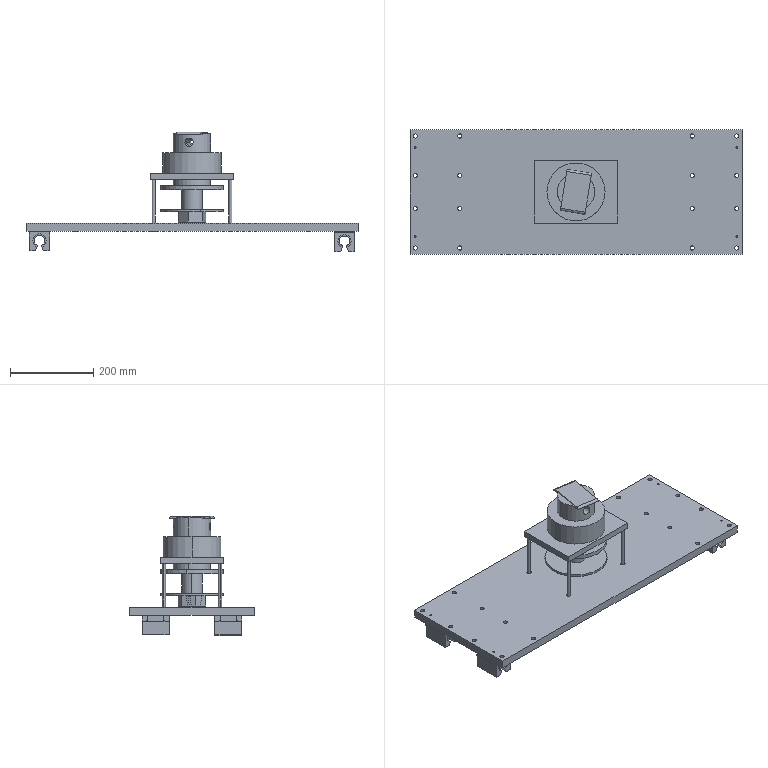Part | SolidWorks | features CompositeCurve 6 | 11 solids | 341 faces | box 800 x 300 x 287.288 mm | volume 7220529 mm3 | cylinder 181 | plane 122 | cone 32 | spline 6 | commonest cylinder face diameters 10 x42 4.2 x40 32 x24 50 x16 25 x12 48 x12